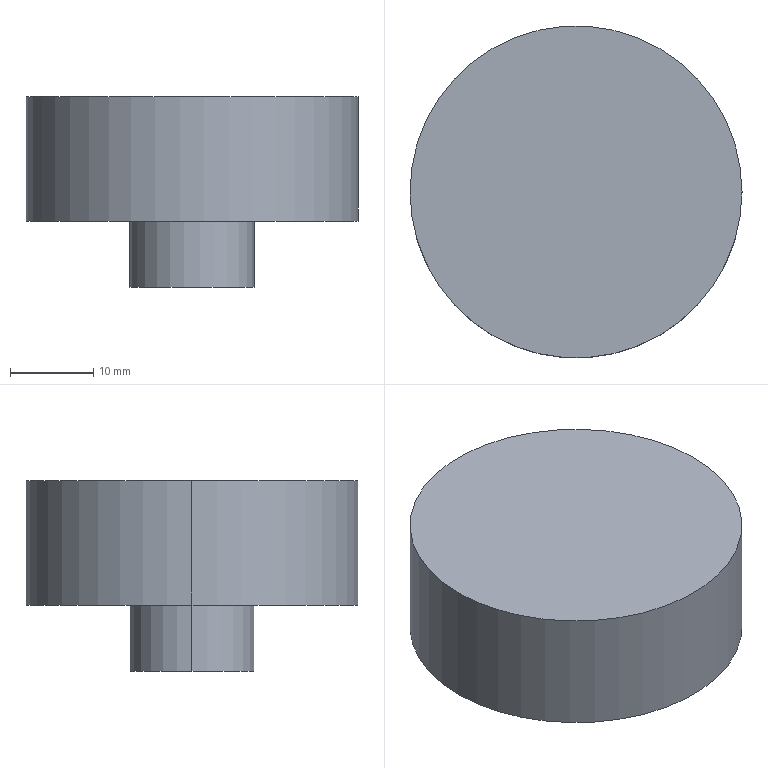Part | STEP file | 1 solid | 7 faces | box 40 x 40 x 23 mm | volume 20263 mm3 | cylinder 4 | plane 3 | commonest cylinder face diameters 15 x2 40 x2
STEP:
#1=CARTESIAN_POINT('',(0.,0.,0.));
#2=DIRECTION('',(0.,0.,1.));
#3=DIRECTION('',(1.,0.,0.));
#4=AXIS2_PLACEMENT_3D('',#1,#2,#3);
#5=CARTESIAN_POINT('',(20.,0.,0.));
#6=VERTEX_POINT('',#5);
#7=CARTESIAN_POINT('',(-20.,0.,0.));
#8=VERTEX_POINT('',#7);
#9=CARTESIAN_POINT('',(0.,0.,0.));
#10=DIRECTION('',(0.,0.,1.));
#11=DIRECTION('',(1.,0.,0.));
#12=AXIS2_PLACEMENT_3D('',#9,#10,#11);
#13=CIRCLE('',#12,20.);
#14=CARTESIAN_POINT('',(0.,0.,15.));
#15=DIRECTION('',(0.,0.,1.));
#16=DIRECTION('',(1.,0.,0.));
#17=AXIS2_PLACEMENT_3D('',#14,#15,#16);
#18=CYLINDRICAL_SURFACE('',#17,20.);
#19=CARTESIAN_POINT('',(0.,-15.));
#20=DIRECTION('',(1.,0.));
#21=VECTOR('',#20,1.);
#22=LINE('',#19,#21);
#23=(GEOMETRIC_REPRESENTATION_CONTEXT(2)PARAMETRIC_REPRESENTATION_CONTEXT()REPRESENTATION_CONTEXT('',''));
#24=DEFINITIONAL_REPRESENTATION('',(#22),#23);
#25=PCURVE('',#18,#24);
#26=CARTESIAN_POINT('',(0.,0.,0.));
#27=DIRECTION('',(0.,0.,1.));
#28=DIRECTION('',(1.,0.,0.));
#29=AXIS2_PLACEMENT_3D('',#26,#27,#28);
#30=PLANE('',#29);
#31=CARTESIAN_POINT('',(0.,0.));
#32=DIRECTION('',(1.,0.));
#33=AXIS2_PLACEMENT_2D('',#31,#32);
#34=CIRCLE('',#33,20.);
#35=(GEOMETRIC_REPRESENTATION_CONTEXT(2)PARAMETRIC_REPRESENTATION_CONTEXT()REPRESENTATION_CONTEXT('',''));
#36=DEFINITIONAL_REPRESENTATION('',(#34),#35);
#37=PCURVE('',#30,#36);
#38=SURFACE_CURVE('',#13,(#25,#37),.PCURVE_S1.);
#39=EDGE_CURVE('',#6,#8,#38,.T.);
#40=ORIENTED_EDGE('',*,*,#39,.T.);
#41=CARTESIAN_POINT('',(-20.,0.,15.));
#42=VERTEX_POINT('',#41);
#43=CARTESIAN_POINT('',(-20.,0.,15.));
#44=DIRECTION('',(0.,0.,1.));
#45=VECTOR('',#44,1.);
#46=LINE('',#43,#45);
#47=CARTESIAN_POINT('',(3.142,0.));
#48=DIRECTION('',(0.,1.));
#49=VECTOR('',#48,1.);
#50=LINE('',#47,#49);
#51=(GEOMETRIC_REPRESENTATION_CONTEXT(2)PARAMETRIC_REPRESENTATION_CONTEXT()REPRESENTATION_CONTEXT('',''));
#52=DEFINITIONAL_REPRESENTATION('',(#50),#51);
#53=PCURVE('',#18,#52);
#54=CARTESIAN_POINT('',(0.,0.,15.));
#55=DIRECTION('',(0.,0.,1.));
#56=DIRECTION('',(1.,0.,0.));
#57=AXIS2_PLACEMENT_3D('',#54,#55,#56);
#58=CYLINDRICAL_SURFACE('',#57,20.);
#59=CARTESIAN_POINT('',(3.142,0.));
#60=DIRECTION('',(0.,1.));
#61=VECTOR('',#60,1.);
#62=LINE('',#59,#61);
#63=(GEOMETRIC_REPRESENTATION_CONTEXT(2)PARAMETRIC_REPRESENTATION_CONTEXT()REPRESENTATION_CONTEXT('',''));
#64=DEFINITIONAL_REPRESENTATION('',(#62),#63);
#65=PCURVE('',#58,#64);
#66=SURFACE_CURVE('',#46,(#53,#65),.PCURVE_S1.);
#67=EDGE_CURVE('',#8,#42,#66,.T.);
#68=ORIENTED_EDGE('',*,*,#67,.T.);
#69=CARTESIAN_POINT('',(20.,0.,15.));
#70=VERTEX_POINT('',#69);
#71=CARTESIAN_POINT('',(0.,0.,15.));
#72=DIRECTION('',(0.,0.,1.));
#73=DIRECTION('',(1.,0.,0.));
#74=AXIS2_PLACEMENT_3D('',#71,#72,#73);
#75=CIRCLE('',#74,20.);
#76=CARTESIAN_POINT('',(0.,0.));
#77=DIRECTION('',(1.,0.));
#78=VECTOR('',#77,1.);
#79=LINE('',#76,#78);
#80=(GEOMETRIC_REPRESENTATION_CONTEXT(2)PARAMETRIC_REPRESENTATION_CONTEXT()REPRESENTATION_CONTEXT('',''));
#81=DEFINITIONAL_REPRESENTATION('',(#79),#80);
#82=PCURVE('',#18,#81);
#83=CARTESIAN_POINT('',(0.,0.,15.));
#84=DIRECTION('',(0.,0.,1.));
#85=DIRECTION('',(1.,0.,0.));
#86=AXIS2_PLACEMENT_3D('',#83,#84,#85);
#87=PLANE('',#86);
#88=CARTESIAN_POINT('',(0.,0.));
#89=DIRECTION('',(1.,0.));
#90=AXIS2_PLACEMENT_2D('',#88,#89);
#91=CIRCLE('',#90,20.);
#92=(GEOMETRIC_REPRESENTATION_CONTEXT(2)PARAMETRIC_REPRESENTATION_CONTEXT()REPRESENTATION_CONTEXT('',''));
#93=DEFINITIONAL_REPRESENTATION('',(#91),#92);
#94=PCURVE('',#87,#93);
#95=SURFACE_CURVE('',#75,(#82,#94),.PCURVE_S1.);
#96=EDGE_CURVE('',#70,#42,#95,.T.);
#97=ORIENTED_EDGE('',*,*,#96,.F.);
#98=CARTESIAN_POINT('',(20.,0.,15.));
#99=DIRECTION('',(0.,0.,1.));
#100=VECTOR('',#99,1.);
#101=LINE('',#98,#100);
#102=CARTESIAN_POINT('',(0.,0.));
#103=DIRECTION('',(0.,1.));
#104=VECTOR('',#103,1.);
#105=LINE('',#102,#104);
#106=(GEOMETRIC_REPRESENTATION_CONTEXT(2)PARAMETRIC_REPRESENTATION_CONTEXT()REPRESENTATION_CONTEXT('',''));
#107=DEFINITIONAL_REPRESENTATION('',(#105),#106);
#108=PCURVE('',#18,#107);
#109=CARTESIAN_POINT('',(6.283,0.));
#110=DIRECTION('',(0.,1.));
#111=VECTOR('',#110,1.);
#112=LINE('',#109,#111);
#113=(GEOMETRIC_REPRESENTATION_CONTEXT(2)PARAMETRIC_REPRESENTATION_CONTEXT()REPRESENTATION_CONTEXT('',''));
#114=DEFINITIONAL_REPRESENTATION('',(#112),#113);
#115=PCURVE('',#58,#114);
#116=SURFACE_CURVE('',#101,(#108,#115),.PCURVE_S1.);
#117=EDGE_CURVE('',#6,#70,#116,.T.);
#118=ORIENTED_EDGE('',*,*,#117,.F.);
#119=EDGE_LOOP('',(#40,#68,#97,#118));
#120=FACE_BOUND('',#119,.T.);
#121=ADVANCED_FACE('',(#120),#18,.T.);
#122=CARTESIAN_POINT('',(-7.5,0.,0.));
#123=VERTEX_POINT('',#122);
#124=CARTESIAN_POINT('',(7.5,0.,0.));
#125=VERTEX_POINT('',#124);
#126=CARTESIAN_POINT('',(0.,0.,0.));
#127=DIRECTION('',(0.,0.,-1.));
#128=DIRECTION('',(-1.,0.,0.));
#129=AXIS2_PLACEMENT_3D('',#126,#127,#128);
#130=CIRCLE('',#129,7.5);
#131=CARTESIAN_POINT('',(0.,0.,-8.));
#132=DIRECTION('',(0.,0.,-1.));
#133=DIRECTION('',(-1.,0.,0.));
#134=AXIS2_PLACEMENT_3D('',#131,#132,#133);
#135=CYLINDRICAL_SURFACE('',#134,7.5);
#136=CARTESIAN_POINT('',(0.,-8.));
#137=DIRECTION('',(1.,0.));
#138=VECTOR('',#137,1.);
#139=LINE('',#136,#138);
#140=(GEOMETRIC_REPRESENTATION_CONTEXT(2)PARAMETRIC_REPRESENTATION_CONTEXT()REPRESENTATION_CONTEXT('',''));
#141=DEFINITIONAL_REPRESENTATION('',(#139),#140);
#142=PCURVE('',#135,#141);
#143=CARTESIAN_POINT('',(-7.5,0.));
#144=CARTESIAN_POINT('',(-7.5,12.99));
#145=CARTESIAN_POINT('',(3.75,6.495));
#146=CARTESIAN_POINT('',(15.,0.));
#147=CARTESIAN_POINT('',(3.75,-6.495));
#148=CARTESIAN_POINT('',(-7.5,-12.99));
#149=CARTESIAN_POINT('',(-7.5,0.));
#150=(BOUNDED_CURVE()B_SPLINE_CURVE(2,(#143,#144,#145,#146,#147,#148,#149),.UNSPECIFIED.,.T.,.F.)B_SPLINE_CURVE_WITH_KNOTS((1,2,2,2,2,1),(-2.094,0.,2.094,4.189,6.283,8.378),.UNSPECIFIED.)CURVE()GEOMETRIC_REPRESENTATION_ITEM()RATIONAL_B_SPLINE_CURVE((1.,0.5,1.,0.5,1.,0.5,1.))REPRESENTATION_ITEM(''));
#151=(GEOMETRIC_REPRESENTATION_CONTEXT(2)PARAMETRIC_REPRESENTATION_CONTEXT()REPRESENTATION_CONTEXT('',''));
#152=DEFINITIONAL_REPRESENTATION('',(#150),#151);
#153=PCURVE('',#30,#152);
#154=SURFACE_CURVE('',#130,(#142,#153),.PCURVE_S1.);
#155=EDGE_CURVE('',#123,#125,#154,.T.);
#156=ORIENTED_EDGE('',*,*,#155,.T.);
#157=CARTESIAN_POINT('',(7.5,0.,-8.));
#158=VERTEX_POINT('',#157);
#159=CARTESIAN_POINT('',(7.5,0.,-8.));
#160=DIRECTION('',(0.,0.,-1.));
#161=VECTOR('',#160,1.);
#162=LINE('',#159,#161);
#163=CARTESIAN_POINT('',(3.142,0.));
#164=DIRECTION('',(0.,1.));
#165=VECTOR('',#164,1.);
#166=LINE('',#163,#165);
#167=(GEOMETRIC_REPRESENTATION_CONTEXT(2)PARAMETRIC_REPRESENTATION_CONTEXT()REPRESENTATION_CONTEXT('',''));
#168=DEFINITIONAL_REPRESENTATION('',(#166),#167);
#169=PCURVE('',#135,#168);
#170=CARTESIAN_POINT('',(0.,0.,-8.));
#171=DIRECTION('',(0.,0.,-1.));
#172=DIRECTION('',(-1.,0.,0.));
#173=AXIS2_PLACEMENT_3D('',#170,#171,#172);
#174=CYLINDRICAL_SURFACE('',#173,7.5);
#175=CARTESIAN_POINT('',(3.142,0.));
#176=DIRECTION('',(0.,1.));
#177=VECTOR('',#176,1.);
#178=LINE('',#175,#177);
#179=(GEOMETRIC_REPRESENTATION_CONTEXT(2)PARAMETRIC_REPRESENTATION_CONTEXT()REPRESENTATION_CONTEXT('',''));
#180=DEFINITIONAL_REPRESENTATION('',(#178),#179);
#181=PCURVE('',#174,#180);
#182=SURFACE_CURVE('',#162,(#169,#181),.PCURVE_S1.);
#183=EDGE_CURVE('',#125,#158,#182,.T.);
#184=ORIENTED_EDGE('',*,*,#183,.T.);
#185=CARTESIAN_POINT('',(-7.5,0.,-8.));
#186=VERTEX_POINT('',#185);
#187=CARTESIAN_POINT('',(0.,0.,-8.));
#188=DIRECTION('',(0.,0.,1.));
#189=DIRECTION('',(-1.,0.,0.));
#190=AXIS2_PLACEMENT_3D('',#187,#188,#189);
#191=CIRCLE('',#190,7.5);
#192=CARTESIAN_POINT('',(6.283,0.));
#193=DIRECTION('',(-1.,0.));
#194=VECTOR('',#193,1.);
#195=LINE('',#192,#194);
#196=(GEOMETRIC_REPRESENTATION_CONTEXT(2)PARAMETRIC_REPRESENTATION_CONTEXT()REPRESENTATION_CONTEXT('',''));
#197=DEFINITIONAL_REPRESENTATION('',(#195),#196);
#198=PCURVE('',#135,#197);
#199=CARTESIAN_POINT('',(0.,0.,-8.));
#200=DIRECTION('',(0.,0.,-1.));
#201=DIRECTION('',(-1.,0.,0.));
#202=AXIS2_PLACEMENT_3D('',#199,#200,#201);
#203=PLANE('',#202);
#204=CARTESIAN_POINT('',(7.5,0.));
#205=CARTESIAN_POINT('',(7.5,-12.99));
#206=CARTESIAN_POINT('',(-3.75,-6.495));
#207=CARTESIAN_POINT('',(-15.,0.));
#208=CARTESIAN_POINT('',(-3.75,6.495));
#209=CARTESIAN_POINT('',(7.5,12.99));
#210=CARTESIAN_POINT('',(7.5,0.));
#211=(BOUNDED_CURVE()B_SPLINE_CURVE(2,(#204,#205,#206,#207,#208,#209,#210),.UNSPECIFIED.,.T.,.F.)B_SPLINE_CURVE_WITH_KNOTS((1,2,2,2,2,1),(-2.094,0.,2.094,4.189,6.283,8.378),.UNSPECIFIED.)CURVE()GEOMETRIC_REPRESENTATION_ITEM()RATIONAL_B_SPLINE_CURVE((1.,0.5,1.,0.5,1.,0.5,1.))REPRESENTATION_ITEM(''));
#212=(GEOMETRIC_REPRESENTATION_CONTEXT(2)PARAMETRIC_REPRESENTATION_CONTEXT()REPRESENTATION_CONTEXT('',''));
#213=DEFINITIONAL_REPRESENTATION('',(#211),#212);
#214=PCURVE('',#203,#213);
#215=SURFACE_CURVE('',#191,(#198,#214),.PCURVE_S1.);
#216=EDGE_CURVE('',#158,#186,#215,.T.);
#217=ORIENTED_EDGE('',*,*,#216,.T.);
#218=CARTESIAN_POINT('',(-7.5,0.,-8.));
#219=DIRECTION('',(0.,0.,-1.));
#220=VECTOR('',#219,1.);
#221=LINE('',#218,#220);
#222=CARTESIAN_POINT('',(0.,0.));
#223=DIRECTION('',(0.,1.));
#224=VECTOR('',#223,1.);
#225=LINE('',#222,#224);
#226=(GEOMETRIC_REPRESENTATION_CONTEXT(2)PARAMETRIC_REPRESENTATION_CONTEXT()REPRESENTATION_CONTEXT('',''));
#227=DEFINITIONAL_REPRESENTATION('',(#225),#226);
#228=PCURVE('',#135,#227);
#229=CARTESIAN_POINT('',(6.283,0.));
#230=DIRECTION('',(0.,1.));
#231=VECTOR('',#230,1.);
#232=LINE('',#229,#231);
#233=(GEOMETRIC_REPRESENTATION_CONTEXT(2)PARAMETRIC_REPRESENTATION_CONTEXT()REPRESENTATION_CONTEXT('',''));
#234=DEFINITIONAL_REPRESENTATION('',(#232),#233);
#235=PCURVE('',#174,#234);
#236=SURFACE_CURVE('',#221,(#228,#235),.PCURVE_S1.);
#237=EDGE_CURVE('',#123,#186,#236,.T.);
#238=ORIENTED_EDGE('',*,*,#237,.F.);
#239=EDGE_LOOP('',(#156,#184,#217,#238));
#240=FACE_BOUND('',#239,.T.);
#241=ADVANCED_FACE('',(#240),#135,.T.);
#242=ORIENTED_EDGE('',*,*,#96,.T.);
#243=CARTESIAN_POINT('',(0.,0.,15.));
#244=DIRECTION('',(0.,0.,1.));
#245=DIRECTION('',(1.,0.,0.));
#246=AXIS2_PLACEMENT_3D('',#243,#244,#245);
#247=CIRCLE('',#246,20.);
#248=CARTESIAN_POINT('',(0.,0.));
#249=DIRECTION('',(1.,0.));
#250=AXIS2_PLACEMENT_2D('',#248,#249);
#251=CIRCLE('',#250,20.);
#252=(GEOMETRIC_REPRESENTATION_CONTEXT(2)PARAMETRIC_REPRESENTATION_CONTEXT()REPRESENTATION_CONTEXT('',''));
#253=DEFINITIONAL_REPRESENTATION('',(#251),#252);
#254=PCURVE('',#87,#253);
#255=CARTESIAN_POINT('',(0.,0.));
#256=DIRECTION('',(1.,0.));
#257=VECTOR('',#256,1.);
#258=LINE('',#255,#257);
#259=(GEOMETRIC_REPRESENTATION_CONTEXT(2)PARAMETRIC_REPRESENTATION_CONTEXT()REPRESENTATION_CONTEXT('',''));
#260=DEFINITIONAL_REPRESENTATION('',(#258),#259);
#261=PCURVE('',#58,#260);
#262=SURFACE_CURVE('',#247,(#254,#261),.PCURVE_S1.);
#263=EDGE_CURVE('',#42,#70,#262,.T.);
#264=ORIENTED_EDGE('',*,*,#263,.T.);
#265=EDGE_LOOP('',(#242,#264));
#266=FACE_BOUND('',#265,.T.);
#267=ADVANCED_FACE('',(#266),#87,.T.);
#268=ORIENTED_EDGE('',*,*,#67,.F.);
#269=CARTESIAN_POINT('',(0.,0.,0.));
#270=DIRECTION('',(0.,0.,1.));
#271=DIRECTION('',(1.,0.,0.));
#272=AXIS2_PLACEMENT_3D('',#269,#270,#271);
#273=CIRCLE('',#272,20.);
#274=CARTESIAN_POINT('',(0.,-15.));
#275=DIRECTION('',(1.,0.));
#276=VECTOR('',#275,1.);
#277=LINE('',#274,#276);
#278=(GEOMETRIC_REPRESENTATION_CONTEXT(2)PARAMETRIC_REPRESENTATION_CONTEXT()REPRESENTATION_CONTEXT('',''));
#279=DEFINITIONAL_REPRESENTATION('',(#277),#278);
#280=PCURVE('',#58,#279);
#281=CARTESIAN_POINT('',(0.,0.));
#282=DIRECTION('',(1.,0.));
#283=AXIS2_PLACEMENT_2D('',#281,#282);
#284=CIRCLE('',#283,20.);
#285=(GEOMETRIC_REPRESENTATION_CONTEXT(2)PARAMETRIC_REPRESENTATION_CONTEXT()REPRESENTATION_CONTEXT('',''));
#286=DEFINITIONAL_REPRESENTATION('',(#284),#285);
#287=PCURVE('',#30,#286);
#288=SURFACE_CURVE('',#273,(#280,#287),.PCURVE_S1.);
#289=EDGE_CURVE('',#8,#6,#288,.T.);
#290=ORIENTED_EDGE('',*,*,#289,.T.);
#291=ORIENTED_EDGE('',*,*,#117,.T.);
#292=ORIENTED_EDGE('',*,*,#263,.F.);
#293=EDGE_LOOP('',(#268,#290,#291,#292));
#294=FACE_BOUND('',#293,.T.);
#295=ADVANCED_FACE('',(#294),#58,.T.);
#296=ORIENTED_EDGE('',*,*,#155,.F.);
#297=CARTESIAN_POINT('',(0.,0.,0.));
#298=DIRECTION('',(0.,0.,-1.));
#299=DIRECTION('',(-1.,0.,0.));
#300=AXIS2_PLACEMENT_3D('',#297,#298,#299);
#301=CIRCLE('',#300,7.5);
#302=CARTESIAN_POINT('',(-7.5,0.));
#303=CARTESIAN_POINT('',(-7.5,12.99));
#304=CARTESIAN_POINT('',(3.75,6.495));
#305=CARTESIAN_POINT('',(15.,0.));
#306=CARTESIAN_POINT('',(3.75,-6.495));
#307=CARTESIAN_POINT('',(-7.5,-12.99));
#308=CARTESIAN_POINT('',(-7.5,0.));
#309=(BOUNDED_CURVE()B_SPLINE_CURVE(2,(#302,#303,#304,#305,#306,#307,#308),.UNSPECIFIED.,.T.,.F.)B_SPLINE_CURVE_WITH_KNOTS((1,2,2,2,2,1),(-2.094,0.,2.094,4.189,6.283,8.378),.UNSPECIFIED.)CURVE()GEOMETRIC_REPRESENTATION_ITEM()RATIONAL_B_SPLINE_CURVE((1.,0.5,1.,0.5,1.,0.5,1.))REPRESENTATION_ITEM(''));
#310=(GEOMETRIC_REPRESENTATION_CONTEXT(2)PARAMETRIC_REPRESENTATION_CONTEXT()REPRESENTATION_CONTEXT('',''));
#311=DEFINITIONAL_REPRESENTATION('',(#309),#310);
#312=PCURVE('',#30,#311);
#313=CARTESIAN_POINT('',(0.,-8.));
#314=DIRECTION('',(1.,0.));
#315=VECTOR('',#314,1.);
#316=LINE('',#313,#315);
#317=(GEOMETRIC_REPRESENTATION_CONTEXT(2)PARAMETRIC_REPRESENTATION_CONTEXT()REPRESENTATION_CONTEXT('',''));
#318=DEFINITIONAL_REPRESENTATION('',(#316),#317);
#319=PCURVE('',#174,#318);
#320=SURFACE_CURVE('',#301,(#312,#319),.PCURVE_S1.);
#321=EDGE_CURVE('',#125,#123,#320,.T.);
#322=ORIENTED_EDGE('',*,*,#321,.F.);
#323=EDGE_LOOP('',(#296,#322));
#324=FACE_BOUND('',#323,.T.);
#325=ORIENTED_EDGE('',*,*,#39,.F.);
#326=ORIENTED_EDGE('',*,*,#289,.F.);
#327=EDGE_LOOP('',(#325,#326));
#328=FACE_BOUND('',#327,.T.);
#329=ADVANCED_FACE('',(#324,#328),#30,.F.);
#330=ORIENTED_EDGE('',*,*,#183,.F.);
#331=ORIENTED_EDGE('',*,*,#321,.T.);
#332=ORIENTED_EDGE('',*,*,#237,.T.);
#333=CARTESIAN_POINT('',(0.,0.,-8.));
#334=DIRECTION('',(0.,0.,1.));
#335=DIRECTION('',(-1.,0.,0.));
#336=AXIS2_PLACEMENT_3D('',#333,#334,#335);
#337=CIRCLE('',#336,7.5);
#338=CARTESIAN_POINT('',(6.283,0.));
#339=DIRECTION('',(-1.,0.));
#340=VECTOR('',#339,1.);
#341=LINE('',#338,#340);
#342=(GEOMETRIC_REPRESENTATION_CONTEXT(2)PARAMETRIC_REPRESENTATION_CONTEXT()REPRESENTATION_CONTEXT('',''));
#343=DEFINITIONAL_REPRESENTATION('',(#341),#342);
#344=PCURVE('',#174,#343);
#345=CARTESIAN_POINT('',(7.5,0.));
#346=CARTESIAN_POINT('',(7.5,-12.99));
#347=CARTESIAN_POINT('',(-3.75,-6.495));
#348=CARTESIAN_POINT('',(-15.,0.));
#349=CARTESIAN_POINT('',(-3.75,6.495));
#350=CARTESIAN_POINT('',(7.5,12.99));
#351=CARTESIAN_POINT('',(7.5,0.));
#352=(BOUNDED_CURVE()B_SPLINE_CURVE(2,(#345,#346,#347,#348,#349,#350,#351),.UNSPECIFIED.,.T.,.F.)B_SPLINE_CURVE_WITH_KNOTS((1,2,2,2,2,1),(-2.094,0.,2.094,4.189,6.283,8.378),.UNSPECIFIED.)CURVE()GEOMETRIC_REPRESENTATION_ITEM()RATIONAL_B_SPLINE_CURVE((1.,0.5,1.,0.5,1.,0.5,1.))REPRESENTATION_ITEM(''));
#353=(GEOMETRIC_REPRESENTATION_CONTEXT(2)PARAMETRIC_REPRESENTATION_CONTEXT()REPRESENTATION_CONTEXT('',''));
#354=DEFINITIONAL_REPRESENTATION('',(#352),#353);
#355=PCURVE('',#203,#354);
#356=SURFACE_CURVE('',#337,(#344,#355),.PCURVE_S1.);
#357=EDGE_CURVE('',#186,#158,#356,.T.);
#358=ORIENTED_EDGE('',*,*,#357,.T.);
#359=EDGE_LOOP('',(#330,#331,#332,#358));
#360=FACE_BOUND('',#359,.T.);
#361=ADVANCED_FACE('',(#360),#174,.T.);
#362=ORIENTED_EDGE('',*,*,#357,.F.);
#363=ORIENTED_EDGE('',*,*,#216,.F.);
#364=EDGE_LOOP('',(#362,#363));
#365=FACE_BOUND('',#364,.T.);
#366=ADVANCED_FACE('',(#365),#203,.T.);
#367=CLOSED_SHELL('',(#121,#241,#267,#295,#329,#361,#366));
#368=MANIFOLD_SOLID_BREP('',#367);
#369=(LENGTH_UNIT()NAMED_UNIT(*)SI_UNIT(.MILLI.,.METRE.));
#370=UNCERTAINTY_MEASURE_WITH_UNIT(LENGTH_MEASURE(0.0000001),#369,'','');
#371=(NAMED_UNIT(*)PLANE_ANGLE_UNIT()SI_UNIT($,.RADIAN.));
#372=(NAMED_UNIT(*)SI_UNIT($,.STERADIAN.)SOLID_ANGLE_UNIT());
#373=(GEOMETRIC_REPRESENTATION_CONTEXT(3)GLOBAL_UNCERTAINTY_ASSIGNED_CONTEXT((#370))GLOBAL_UNIT_ASSIGNED_CONTEXT((#369,#371,#372))REPRESENTATION_CONTEXT('',''));
#374=ADVANCED_BREP_SHAPE_REPRESENTATION('',(#4,#368),#373);